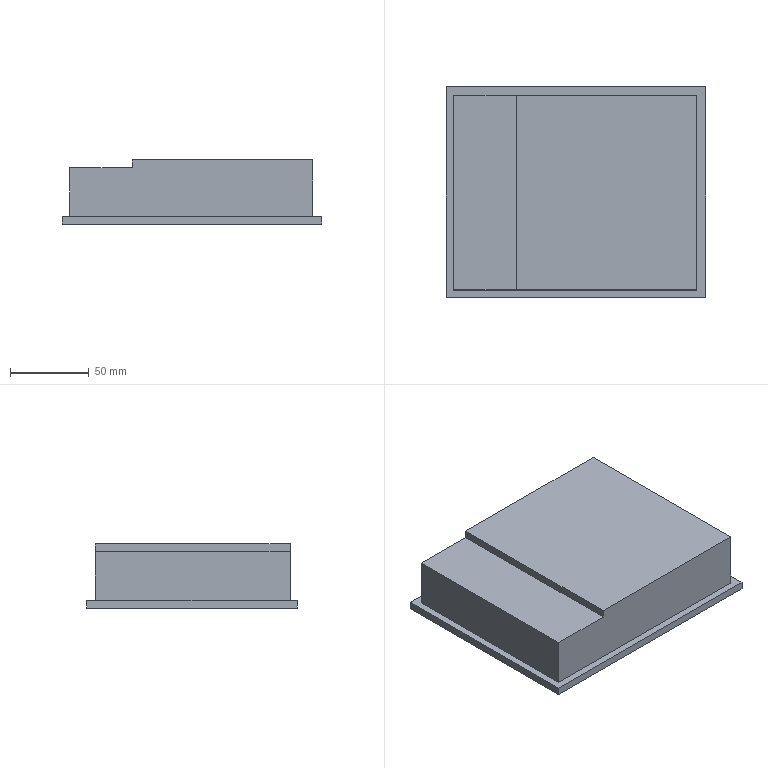Part | STEP file | Display-724_Default | 1 solid | 18 faces | box 165 x 134 x 41 mm | volume 776017 mm3 | plane 18
STEP:
#1=CARTESIAN_POINT('',(0.,0.,0.));
#2=DIRECTION('',(0.,0.,1.));
#3=DIRECTION('',(1.,0.,0.));
#4=AXIS2_PLACEMENT_3D('',#1,#2,#3);
#5=CARTESIAN_POINT('',(-69.492,78.011,5.));
#6=VERTEX_POINT('',#5);
#7=CARTESIAN_POINT('',(-69.492,-55.989,5.));
#8=VERTEX_POINT('',#7);
#9=CARTESIAN_POINT('',(-69.492,78.011,5.));
#10=DIRECTION('',(-0.00000053,-1.,0.));
#11=VECTOR('',#10,1.);
#12=LINE('',#9,#11);
#13=CARTESIAN_POINT('',(-69.492,-55.989,5.));
#14=DIRECTION('',(0.,0.,1.));
#15=DIRECTION('',(1.,0.,0.));
#16=AXIS2_PLACEMENT_3D('',#13,#14,#15);
#17=PLANE('',#16);
#18=CARTESIAN_POINT('',(0.00007096,134.));
#19=DIRECTION('',(-0.00000053,-1.));
#20=VECTOR('',#19,1.);
#21=LINE('',#18,#20);
#22=(GEOMETRIC_REPRESENTATION_CONTEXT(2)PARAMETRIC_REPRESENTATION_CONTEXT()REPRESENTATION_CONTEXT('',''));
#23=DEFINITIONAL_REPRESENTATION('',(#21),#22);
#24=PCURVE('',#17,#23);
#25=CARTESIAN_POINT('',(-69.492,78.011,5.));
#26=DIRECTION('',(1.,-0.00000053,0.));
#27=DIRECTION('',(0.00000053,1.,0.));
#28=AXIS2_PLACEMENT_3D('',#25,#26,#27);
#29=PLANE('',#28);
#30=CARTESIAN_POINT('',(0.,0.));
#31=DIRECTION('',(-1.,0.));
#32=VECTOR('',#31,1.);
#33=LINE('',#30,#32);
#34=(GEOMETRIC_REPRESENTATION_CONTEXT(2)PARAMETRIC_REPRESENTATION_CONTEXT()REPRESENTATION_CONTEXT('',''));
#35=DEFINITIONAL_REPRESENTATION('',(#33),#34);
#36=PCURVE('',#29,#35);
#37=SURFACE_CURVE('',#12,(#24,#36),.PCURVE_S1.);
#38=EDGE_CURVE('',#6,#8,#37,.T.);
#39=ORIENTED_EDGE('',*,*,#38,.T.);
#40=CARTESIAN_POINT('',(95.508,-55.989,5.));
#41=VERTEX_POINT('',#40);
#42=CARTESIAN_POINT('',(-69.492,-55.989,5.));
#43=DIRECTION('',(1.,0.00000006,0.));
#44=VECTOR('',#43,1.);
#45=LINE('',#42,#44);
#46=CARTESIAN_POINT('',(0.,0.));
#47=DIRECTION('',(1.,0.00000006));
#48=VECTOR('',#47,1.);
#49=LINE('',#46,#48);
#50=(GEOMETRIC_REPRESENTATION_CONTEXT(2)PARAMETRIC_REPRESENTATION_CONTEXT()REPRESENTATION_CONTEXT('',''));
#51=DEFINITIONAL_REPRESENTATION('',(#49),#50);
#52=PCURVE('',#17,#51);
#53=CARTESIAN_POINT('',(-69.492,-55.989,5.));
#54=DIRECTION('',(-0.00000006,1.,0.));
#55=DIRECTION('',(-1.,-0.00000006,0.));
#56=AXIS2_PLACEMENT_3D('',#53,#54,#55);
#57=PLANE('',#56);
#58=CARTESIAN_POINT('',(0.,0.));
#59=DIRECTION('',(-1.,0.));
#60=VECTOR('',#59,1.);
#61=LINE('',#58,#60);
#62=(GEOMETRIC_REPRESENTATION_CONTEXT(2)PARAMETRIC_REPRESENTATION_CONTEXT()REPRESENTATION_CONTEXT('',''));
#63=DEFINITIONAL_REPRESENTATION('',(#61),#62);
#64=PCURVE('',#57,#63);
#65=SURFACE_CURVE('',#45,(#52,#64),.PCURVE_S1.);
#66=EDGE_CURVE('',#8,#41,#65,.T.);
#67=ORIENTED_EDGE('',*,*,#66,.T.);
#68=CARTESIAN_POINT('',(95.508,78.011,5.));
#69=VERTEX_POINT('',#68);
#70=CARTESIAN_POINT('',(95.508,78.011,5.));
#71=DIRECTION('',(0.00000053,1.,0.));
#72=VECTOR('',#71,1.);
#73=LINE('',#70,#72);
#74=CARTESIAN_POINT('',(165.,134.));
#75=DIRECTION('',(0.00000053,1.));
#76=VECTOR('',#75,1.);
#77=LINE('',#74,#76);
#78=(GEOMETRIC_REPRESENTATION_CONTEXT(2)PARAMETRIC_REPRESENTATION_CONTEXT()REPRESENTATION_CONTEXT('',''));
#79=DEFINITIONAL_REPRESENTATION('',(#77),#78);
#80=PCURVE('',#17,#79);
#81=CARTESIAN_POINT('',(95.508,78.011,5.));
#82=DIRECTION('',(-1.,0.00000053,0.));
#83=DIRECTION('',(-0.00000053,-1.,0.));
#84=AXIS2_PLACEMENT_3D('',#81,#82,#83);
#85=PLANE('',#84);
#86=CARTESIAN_POINT('',(0.,0.));
#87=DIRECTION('',(-1.,0.));
#88=VECTOR('',#87,1.);
#89=LINE('',#86,#88);
#90=(GEOMETRIC_REPRESENTATION_CONTEXT(2)PARAMETRIC_REPRESENTATION_CONTEXT()REPRESENTATION_CONTEXT('',''));
#91=DEFINITIONAL_REPRESENTATION('',(#89),#90);
#92=PCURVE('',#85,#91);
#93=SURFACE_CURVE('',#73,(#80,#92),.PCURVE_S1.);
#94=EDGE_CURVE('',#41,#69,#93,.T.);
#95=ORIENTED_EDGE('',*,*,#94,.T.);
#96=CARTESIAN_POINT('',(-69.492,78.011,5.));
#97=DIRECTION('',(-1.,-0.00000006,0.));
#98=VECTOR('',#97,1.);
#99=LINE('',#96,#98);
#100=CARTESIAN_POINT('',(0.00007096,134.));
#101=DIRECTION('',(-1.,-0.00000006));
#102=VECTOR('',#101,1.);
#103=LINE('',#100,#102);
#104=(GEOMETRIC_REPRESENTATION_CONTEXT(2)PARAMETRIC_REPRESENTATION_CONTEXT()REPRESENTATION_CONTEXT('',''));
#105=DEFINITIONAL_REPRESENTATION('',(#103),#104);
#106=PCURVE('',#17,#105);
#107=CARTESIAN_POINT('',(-69.492,78.011,5.));
#108=DIRECTION('',(0.00000006,-1.,0.));
#109=DIRECTION('',(1.,0.00000006,0.));
#110=AXIS2_PLACEMENT_3D('',#107,#108,#109);
#111=PLANE('',#110);
#112=CARTESIAN_POINT('',(0.,0.));
#113=DIRECTION('',(-1.,0.));
#114=VECTOR('',#113,1.);
#115=LINE('',#112,#114);
#116=(GEOMETRIC_REPRESENTATION_CONTEXT(2)PARAMETRIC_REPRESENTATION_CONTEXT()REPRESENTATION_CONTEXT('',''));
#117=DEFINITIONAL_REPRESENTATION('',(#115),#116);
#118=PCURVE('',#111,#117);
#119=SURFACE_CURVE('',#99,(#106,#118),.PCURVE_S1.);
#120=EDGE_CURVE('',#69,#6,#119,.T.);
#121=ORIENTED_EDGE('',*,*,#120,.T.);
#122=EDGE_LOOP('',(#39,#67,#95,#121));
#123=FACE_BOUND('',#122,.T.);
#124=CARTESIAN_POINT('',(90.052,72.554,5.));
#125=VERTEX_POINT('',#124);
#126=CARTESIAN_POINT('',(-64.948,72.554,5.));
#127=VERTEX_POINT('',#126);
#128=CARTESIAN_POINT('',(-64.948,72.554,5.));
#129=DIRECTION('',(-1.,0.,0.));
#130=VECTOR('',#129,1.);
#131=LINE('',#128,#130);
#132=CARTESIAN_POINT('',(4.544,128.543));
#133=DIRECTION('',(-1.,0.));
#134=VECTOR('',#133,1.);
#135=LINE('',#132,#134);
#136=(GEOMETRIC_REPRESENTATION_CONTEXT(2)PARAMETRIC_REPRESENTATION_CONTEXT()REPRESENTATION_CONTEXT('',''));
#137=DEFINITIONAL_REPRESENTATION('',(#135),#136);
#138=PCURVE('',#17,#137);
#139=CARTESIAN_POINT('',(-64.948,72.554,41.));
#140=DIRECTION('',(0.,-1.,0.));
#141=DIRECTION('',(0.,0.,-1.));
#142=AXIS2_PLACEMENT_3D('',#139,#140,#141);
#143=PLANE('',#142);
#144=CARTESIAN_POINT('',(36.,0.));
#145=DIRECTION('',(0.,-1.));
#146=VECTOR('',#145,1.);
#147=LINE('',#144,#146);
#148=(GEOMETRIC_REPRESENTATION_CONTEXT(2)PARAMETRIC_REPRESENTATION_CONTEXT()REPRESENTATION_CONTEXT('',''));
#149=DEFINITIONAL_REPRESENTATION('',(#147),#148);
#150=PCURVE('',#143,#149);
#151=SURFACE_CURVE('',#131,(#138,#150),.PCURVE_S1.);
#152=EDGE_CURVE('',#125,#127,#151,.T.);
#153=ORIENTED_EDGE('',*,*,#152,.F.);
#154=CARTESIAN_POINT('',(90.052,-51.446,5.));
#155=VERTEX_POINT('',#154);
#156=CARTESIAN_POINT('',(90.052,72.554,5.));
#157=DIRECTION('',(0.,1.,0.));
#158=VECTOR('',#157,1.);
#159=LINE('',#156,#158);
#160=CARTESIAN_POINT('',(159.544,128.543));
#161=DIRECTION('',(0.,1.));
#162=VECTOR('',#161,1.);
#163=LINE('',#160,#162);
#164=(GEOMETRIC_REPRESENTATION_CONTEXT(2)PARAMETRIC_REPRESENTATION_CONTEXT()REPRESENTATION_CONTEXT('',''));
#165=DEFINITIONAL_REPRESENTATION('',(#163),#164);
#166=PCURVE('',#17,#165);
#167=CARTESIAN_POINT('',(90.052,72.554,41.));
#168=DIRECTION('',(-1.,0.,0.));
#169=DIRECTION('',(0.,-1.,0.));
#170=AXIS2_PLACEMENT_3D('',#167,#168,#169);
#171=PLANE('',#170);
#172=CARTESIAN_POINT('',(0.,-36.));
#173=DIRECTION('',(-1.,0.));
#174=VECTOR('',#173,1.);
#175=LINE('',#172,#174);
#176=(GEOMETRIC_REPRESENTATION_CONTEXT(2)PARAMETRIC_REPRESENTATION_CONTEXT()REPRESENTATION_CONTEXT('',''));
#177=DEFINITIONAL_REPRESENTATION('',(#175),#176);
#178=PCURVE('',#171,#177);
#179=SURFACE_CURVE('',#159,(#166,#178),.PCURVE_S1.);
#180=EDGE_CURVE('',#155,#125,#179,.T.);
#181=ORIENTED_EDGE('',*,*,#180,.F.);
#182=CARTESIAN_POINT('',(-64.948,-51.446,5.));
#183=VERTEX_POINT('',#182);
#184=CARTESIAN_POINT('',(-64.948,-51.446,5.));
#185=DIRECTION('',(1.,0.,0.));
#186=VECTOR('',#185,1.);
#187=LINE('',#184,#186);
#188=CARTESIAN_POINT('',(4.544,4.543));
#189=DIRECTION('',(1.,0.));
#190=VECTOR('',#189,1.);
#191=LINE('',#188,#190);
#192=(GEOMETRIC_REPRESENTATION_CONTEXT(2)PARAMETRIC_REPRESENTATION_CONTEXT()REPRESENTATION_CONTEXT('',''));
#193=DEFINITIONAL_REPRESENTATION('',(#191),#192);
#194=PCURVE('',#17,#193);
#195=CARTESIAN_POINT('',(-64.948,-51.446,41.));
#196=DIRECTION('',(0.,1.,0.));
#197=DIRECTION('',(0.,0.,1.));
#198=AXIS2_PLACEMENT_3D('',#195,#196,#197);
#199=PLANE('',#198);
#200=CARTESIAN_POINT('',(-36.,0.));
#201=DIRECTION('',(0.,1.));
#202=VECTOR('',#201,1.);
#203=LINE('',#200,#202);
#204=(GEOMETRIC_REPRESENTATION_CONTEXT(2)PARAMETRIC_REPRESENTATION_CONTEXT()REPRESENTATION_CONTEXT('',''));
#205=DEFINITIONAL_REPRESENTATION('',(#203),#204);
#206=PCURVE('',#199,#205);
#207=SURFACE_CURVE('',#187,(#194,#206),.PCURVE_S1.);
#208=EDGE_CURVE('',#183,#155,#207,.T.);
#209=ORIENTED_EDGE('',*,*,#208,.F.);
#210=CARTESIAN_POINT('',(-64.948,72.554,5.));
#211=DIRECTION('',(0.,-1.,0.));
#212=VECTOR('',#211,1.);
#213=LINE('',#210,#212);
#214=CARTESIAN_POINT('',(4.544,128.543));
#215=DIRECTION('',(0.,-1.));
#216=VECTOR('',#215,1.);
#217=LINE('',#214,#216);
#218=(GEOMETRIC_REPRESENTATION_CONTEXT(2)PARAMETRIC_REPRESENTATION_CONTEXT()REPRESENTATION_CONTEXT('',''));
#219=DEFINITIONAL_REPRESENTATION('',(#217),#218);
#220=PCURVE('',#17,#219);
#221=CARTESIAN_POINT('',(-64.948,72.554,41.));
#222=DIRECTION('',(1.,0.,0.));
#223=DIRECTION('',(0.,1.,0.));
#224=AXIS2_PLACEMENT_3D('',#221,#222,#223);
#225=PLANE('',#224);
#226=CARTESIAN_POINT('',(0.,-36.));
#227=DIRECTION('',(-1.,0.));
#228=VECTOR('',#227,1.);
#229=LINE('',#226,#228);
#230=(GEOMETRIC_REPRESENTATION_CONTEXT(2)PARAMETRIC_REPRESENTATION_CONTEXT()REPRESENTATION_CONTEXT('',''));
#231=DEFINITIONAL_REPRESENTATION('',(#229),#230);
#232=PCURVE('',#225,#231);
#233=SURFACE_CURVE('',#213,(#220,#232),.PCURVE_S1.);
#234=EDGE_CURVE('',#127,#183,#233,.T.);
#235=ORIENTED_EDGE('',*,*,#234,.F.);
#236=EDGE_LOOP('',(#153,#181,#209,#235));
#237=FACE_BOUND('',#236,.T.);
#238=ADVANCED_FACE('',(#123,#237),#17,.T.);
#239=CARTESIAN_POINT('',(-69.492,78.011,0.));
#240=VERTEX_POINT('',#239);
#241=CARTESIAN_POINT('',(-69.492,-55.989,0.));
#242=VERTEX_POINT('',#241);
#243=CARTESIAN_POINT('',(-69.492,78.011,0.));
#244=DIRECTION('',(-0.00000053,-1.,0.));
#245=VECTOR('',#244,1.);
#246=LINE('',#243,#245);
#247=CARTESIAN_POINT('',(0.,-5.));
#248=DIRECTION('',(-1.,0.));
#249=VECTOR('',#248,1.);
#250=LINE('',#247,#249);
#251=(GEOMETRIC_REPRESENTATION_CONTEXT(2)PARAMETRIC_REPRESENTATION_CONTEXT()REPRESENTATION_CONTEXT('',''));
#252=DEFINITIONAL_REPRESENTATION('',(#250),#251);
#253=PCURVE('',#29,#252);
#254=CARTESIAN_POINT('',(-69.492,-55.989,0.));
#255=DIRECTION('',(0.,0.,1.));
#256=DIRECTION('',(1.,0.,0.));
#257=AXIS2_PLACEMENT_3D('',#254,#255,#256);
#258=PLANE('',#257);
#259=CARTESIAN_POINT('',(0.00007096,134.));
#260=DIRECTION('',(-0.00000053,-1.));
#261=VECTOR('',#260,1.);
#262=LINE('',#259,#261);
#263=(GEOMETRIC_REPRESENTATION_CONTEXT(2)PARAMETRIC_REPRESENTATION_CONTEXT()REPRESENTATION_CONTEXT('',''));
#264=DEFINITIONAL_REPRESENTATION('',(#262),#263);
#265=PCURVE('',#258,#264);
#266=SURFACE_CURVE('',#246,(#253,#265),.PCURVE_S1.);
#267=EDGE_CURVE('',#240,#242,#266,.T.);
#268=ORIENTED_EDGE('',*,*,#267,.T.);
#269=CARTESIAN_POINT('',(-69.492,-55.989,5.));
#270=DIRECTION('',(0.,0.,-1.));
#271=VECTOR('',#270,1.);
#272=LINE('',#269,#271);
#273=CARTESIAN_POINT('',(-134.,0.));
#274=DIRECTION('',(0.,-1.));
#275=VECTOR('',#274,1.);
#276=LINE('',#273,#275);
#277=(GEOMETRIC_REPRESENTATION_CONTEXT(2)PARAMETRIC_REPRESENTATION_CONTEXT()REPRESENTATION_CONTEXT('',''));
#278=DEFINITIONAL_REPRESENTATION('',(#276),#277);
#279=PCURVE('',#29,#278);
#280=CARTESIAN_POINT('',(0.,0.));
#281=DIRECTION('',(0.,-1.));
#282=VECTOR('',#281,1.);
#283=LINE('',#280,#282);
#284=(GEOMETRIC_REPRESENTATION_CONTEXT(2)PARAMETRIC_REPRESENTATION_CONTEXT()REPRESENTATION_CONTEXT('',''));
#285=DEFINITIONAL_REPRESENTATION('',(#283),#284);
#286=PCURVE('',#57,#285);
#287=SURFACE_CURVE('',#272,(#279,#286),.PCURVE_S1.);
#288=EDGE_CURVE('',#8,#242,#287,.T.);
#289=ORIENTED_EDGE('',*,*,#288,.F.);
#290=ORIENTED_EDGE('',*,*,#38,.F.);
#291=CARTESIAN_POINT('',(-69.492,78.011,5.));
#292=DIRECTION('',(0.,0.,-1.));
#293=VECTOR('',#292,1.);
#294=LINE('',#291,#293);
#295=CARTESIAN_POINT('',(0.,0.));
#296=DIRECTION('',(0.,-1.));
#297=VECTOR('',#296,1.);
#298=LINE('',#295,#297);
#299=(GEOMETRIC_REPRESENTATION_CONTEXT(2)PARAMETRIC_REPRESENTATION_CONTEXT()REPRESENTATION_CONTEXT('',''));
#300=DEFINITIONAL_REPRESENTATION('',(#298),#299);
#301=PCURVE('',#29,#300);
#302=CARTESIAN_POINT('',(0.,0.));
#303=DIRECTION('',(0.,-1.));
#304=VECTOR('',#303,1.);
#305=LINE('',#302,#304);
#306=(GEOMETRIC_REPRESENTATION_CONTEXT(2)PARAMETRIC_REPRESENTATION_CONTEXT()REPRESENTATION_CONTEXT('',''));
#307=DEFINITIONAL_REPRESENTATION('',(#305),#306);
#308=PCURVE('',#111,#307);
#309=SURFACE_CURVE('',#294,(#301,#308),.PCURVE_S1.);
#310=EDGE_CURVE('',#6,#240,#309,.T.);
#311=ORIENTED_EDGE('',*,*,#310,.T.);
#312=EDGE_LOOP('',(#268,#289,#290,#311));
#313=FACE_BOUND('',#312,.T.);
#314=ADVANCED_FACE('',(#313),#29,.F.);
#315=CARTESIAN_POINT('',(95.508,-55.989,0.));
#316=VERTEX_POINT('',#315);
#317=CARTESIAN_POINT('',(-69.492,-55.989,0.));
#318=DIRECTION('',(1.,0.00000006,0.));
#319=VECTOR('',#318,1.);
#320=LINE('',#317,#319);
#321=CARTESIAN_POINT('',(0.,-5.));
#322=DIRECTION('',(-1.,0.));
#323=VECTOR('',#322,1.);
#324=LINE('',#321,#323);
#325=(GEOMETRIC_REPRESENTATION_CONTEXT(2)PARAMETRIC_REPRESENTATION_CONTEXT()REPRESENTATION_CONTEXT('',''));
#326=DEFINITIONAL_REPRESENTATION('',(#324),#325);
#327=PCURVE('',#57,#326);
#328=CARTESIAN_POINT('',(0.,0.));
#329=DIRECTION('',(1.,0.00000006));
#330=VECTOR('',#329,1.);
#331=LINE('',#328,#330);
#332=(GEOMETRIC_REPRESENTATION_CONTEXT(2)PARAMETRIC_REPRESENTATION_CONTEXT()REPRESENTATION_CONTEXT('',''));
#333=DEFINITIONAL_REPRESENTATION('',(#331),#332);
#334=PCURVE('',#258,#333);
#335=SURFACE_CURVE('',#320,(#327,#334),.PCURVE_S1.);
#336=EDGE_CURVE('',#242,#316,#335,.T.);
#337=ORIENTED_EDGE('',*,*,#336,.T.);
#338=CARTESIAN_POINT('',(95.508,-55.989,5.));
#339=DIRECTION('',(0.,0.,-1.));
#340=VECTOR('',#339,1.);
#341=LINE('',#338,#340);
#342=CARTESIAN_POINT('',(-165.,0.));
#343=DIRECTION('',(0.,-1.));
#344=VECTOR('',#343,1.);
#345=LINE('',#342,#344);
#346=(GEOMETRIC_REPRESENTATION_CONTEXT(2)PARAMETRIC_REPRESENTATION_CONTEXT()REPRESENTATION_CONTEXT('',''));
#347=DEFINITIONAL_REPRESENTATION('',(#345),#346);
#348=PCURVE('',#57,#347);
#349=CARTESIAN_POINT('',(134.,0.));
#350=DIRECTION('',(0.,-1.));
#351=VECTOR('',#350,1.);
#352=LINE('',#349,#351);
#353=(GEOMETRIC_REPRESENTATION_CONTEXT(2)PARAMETRIC_REPRESENTATION_CONTEXT()REPRESENTATION_CONTEXT('',''));
#354=DEFINITIONAL_REPRESENTATION('',(#352),#353);
#355=PCURVE('',#85,#354);
#356=SURFACE_CURVE('',#341,(#348,#355),.PCURVE_S1.);
#357=EDGE_CURVE('',#41,#316,#356,.T.);
#358=ORIENTED_EDGE('',*,*,#357,.F.);
#359=ORIENTED_EDGE('',*,*,#66,.F.);
#360=ORIENTED_EDGE('',*,*,#288,.T.);
#361=EDGE_LOOP('',(#337,#358,#359,#360));
#362=FACE_BOUND('',#361,.T.);
#363=ADVANCED_FACE('',(#362),#57,.F.);
#364=CARTESIAN_POINT('',(95.508,78.011,0.));
#365=VERTEX_POINT('',#364);
#366=CARTESIAN_POINT('',(95.508,78.011,0.));
#367=DIRECTION('',(0.00000053,1.,0.));
#368=VECTOR('',#367,1.);
#369=LINE('',#366,#368);
#370=CARTESIAN_POINT('',(0.,-5.));
#371=DIRECTION('',(-1.,0.));
#372=VECTOR('',#371,1.);
#373=LINE('',#370,#372);
#374=(GEOMETRIC_REPRESENTATION_CONTEXT(2)PARAMETRIC_REPRESENTATION_CONTEXT()REPRESENTATION_CONTEXT('',''));
#375=DEFINITIONAL_REPRESENTATION('',(#373),#374);
#376=PCURVE('',#85,#375);
#377=CARTESIAN_POINT('',(165.,134.));
#378=DIRECTION('',(0.00000053,1.));
#379=VECTOR('',#378,1.);
#380=LINE('',#377,#379);
#381=(GEOMETRIC_REPRESENTATION_CONTEXT(2)PARAMETRIC_REPRESENTATION_CONTEXT()REPRESENTATION_CONTEXT('',''));
#382=DEFINITIONAL_REPRESENTATION('',(#380),#381);
#383=PCURVE('',#258,#382);
#384=SURFACE_CURVE('',#369,(#376,#383),.PCURVE_S1.);
#385=EDGE_CURVE('',#316,#365,#384,.T.);
#386=ORIENTED_EDGE('',*,*,#385,.T.);
#387=CARTESIAN_POINT('',(95.508,78.011,5.));
#388=DIRECTION('',(0.,0.,-1.));
#389=VECTOR('',#388,1.);
#390=LINE('',#387,#389);
#391=CARTESIAN_POINT('',(0.,0.));
#392=DIRECTION('',(0.,-1.));
#393=VECTOR('',#392,1.);
#394=LINE('',#391,#393);
#395=(GEOMETRIC_REPRESENTATION_CONTEXT(2)PARAMETRIC_REPRESENTATION_CONTEXT()REPRESENTATION_CONTEXT('',''));
#396=DEFINITIONAL_REPRESENTATION('',(#394),#395);
#397=PCURVE('',#85,#396);
#398=CARTESIAN_POINT('',(165.,0.));
#399=DIRECTION('',(0.,-1.));
#400=VECTOR('',#399,1.);
#401=LINE('',#398,#400);
#402=(GEOMETRIC_REPRESENTATION_CONTEXT(2)PARAMETRIC_REPRESENTATION_CONTEXT()REPRESENTATION_CONTEXT('',''));
#403=DEFINITIONAL_REPRESENTATION('',(#401),#402);
#404=PCURVE('',#111,#403);
#405=SURFACE_CURVE('',#390,(#397,#404),.PCURVE_S1.);
#406=EDGE_CURVE('',#69,#365,#405,.T.);
#407=ORIENTED_EDGE('',*,*,#406,.F.);
#408=ORIENTED_EDGE('',*,*,#94,.F.);
#409=ORIENTED_EDGE('',*,*,#357,.T.);
#410=EDGE_LOOP('',(#386,#407,#408,#409));
#411=FACE_BOUND('',#410,.T.);
#412=ADVANCED_FACE('',(#411),#85,.F.);
#413=CARTESIAN_POINT('',(-69.492,78.011,0.));
#414=DIRECTION('',(-1.,-0.00000006,0.));
#415=VECTOR('',#414,1.);
#416=LINE('',#413,#415);
#417=CARTESIAN_POINT('',(0.,-5.));
#418=DIRECTION('',(-1.,0.));
#419=VECTOR('',#418,1.);
#420=LINE('',#417,#419);
#421=(GEOMETRIC_REPRESENTATION_CONTEXT(2)PARAMETRIC_REPRESENTATION_CONTEXT()REPRESENTATION_CONTEXT('',''));
#422=DEFINITIONAL_REPRESENTATION('',(#420),#421);
#423=PCURVE('',#111,#422);
#424=CARTESIAN_POINT('',(0.00007096,134.));
#425=DIRECTION('',(-1.,-0.00000006));
#426=VECTOR('',#425,1.);
#427=LINE('',#424,#426);
#428=(GEOMETRIC_REPRESENTATION_CONTEXT(2)PARAMETRIC_REPRESENTATION_CONTEXT()REPRESENTATION_CONTEXT('',''));
#429=DEFINITIONAL_REPRESENTATION('',(#427),#428);
#430=PCURVE('',#258,#429);
#431=SURFACE_CURVE('',#416,(#423,#430),.PCURVE_S1.);
#432=EDGE_CURVE('',#365,#240,#431,.T.);
#433=ORIENTED_EDGE('',*,*,#432,.T.);
#434=ORIENTED_EDGE('',*,*,#310,.F.);
#435=ORIENTED_EDGE('',*,*,#120,.F.);
#436=ORIENTED_EDGE('',*,*,#406,.T.);
#437=EDGE_LOOP('',(#433,#434,#435,#436));
#438=FACE_BOUND('',#437,.T.);
#439=ADVANCED_FACE('',(#438),#111,.F.);
#440=CARTESIAN_POINT('',(85.508,-45.989,0.));
#441=VERTEX_POINT('',#440);
#442=CARTESIAN_POINT('',(-59.492,-45.989,0.));
#443=VERTEX_POINT('',#442);
#444=CARTESIAN_POINT('',(85.508,-45.989,0.));
#445=DIRECTION('',(-1.,-0.00000006,0.));
#446=VECTOR('',#445,1.);
#447=LINE('',#444,#446);
#448=CARTESIAN_POINT('',(155.,10.));
#449=DIRECTION('',(-1.,-0.00000006));
#450=VECTOR('',#449,1.);
#451=LINE('',#448,#450);
#452=(GEOMETRIC_REPRESENTATION_CONTEXT(2)PARAMETRIC_REPRESENTATION_CONTEXT()REPRESENTATION_CONTEXT('',''));
#453=DEFINITIONAL_REPRESENTATION('',(#451),#452);
#454=PCURVE('',#258,#453);
#455=CARTESIAN_POINT('',(85.508,-45.989,0.1));
#456=DIRECTION('',(0.00000006,-1.,0.));
#457=DIRECTION('',(1.,0.00000006,0.));
#458=AXIS2_PLACEMENT_3D('',#455,#456,#457);
#459=PLANE('',#458);
#460=CARTESIAN_POINT('',(0.,-0.1));
#461=DIRECTION('',(-1.,0.));
#462=VECTOR('',#461,1.);
#463=LINE('',#460,#462);
#464=(GEOMETRIC_REPRESENTATION_CONTEXT(2)PARAMETRIC_REPRESENTATION_CONTEXT()REPRESENTATION_CONTEXT('',''));
#465=DEFINITIONAL_REPRESENTATION('',(#463),#464);
#466=PCURVE('',#459,#465);
#467=SURFACE_CURVE('',#447,(#454,#466),.PCURVE_S1.);
#468=EDGE_CURVE('',#441,#443,#467,.T.);
#469=ORIENTED_EDGE('',*,*,#468,.F.);
#470=CARTESIAN_POINT('',(85.508,68.011,0.));
#471=VERTEX_POINT('',#470);
#472=CARTESIAN_POINT('',(85.508,68.011,0.));
#473=DIRECTION('',(-0.00000053,-1.,0.));
#474=VECTOR('',#473,1.);
#475=LINE('',#472,#474);
#476=CARTESIAN_POINT('',(155.,124.));
#477=DIRECTION('',(-0.00000053,-1.));
#478=VECTOR('',#477,1.);
#479=LINE('',#476,#478);
#480=(GEOMETRIC_REPRESENTATION_CONTEXT(2)PARAMETRIC_REPRESENTATION_CONTEXT()REPRESENTATION_CONTEXT('',''));
#481=DEFINITIONAL_REPRESENTATION('',(#479),#480);
#482=PCURVE('',#258,#481);
#483=CARTESIAN_POINT('',(85.508,68.011,0.1));
#484=DIRECTION('',(1.,-0.00000053,0.));
#485=DIRECTION('',(0.00000053,1.,0.));
#486=AXIS2_PLACEMENT_3D('',#483,#484,#485);
#487=PLANE('',#486);
#488=CARTESIAN_POINT('',(0.,-0.1));
#489=DIRECTION('',(-1.,0.));
#490=VECTOR('',#489,1.);
#491=LINE('',#488,#490);
#492=(GEOMETRIC_REPRESENTATION_CONTEXT(2)PARAMETRIC_REPRESENTATION_CONTEXT()REPRESENTATION_CONTEXT('',''));
#493=DEFINITIONAL_REPRESENTATION('',(#491),#492);
#494=PCURVE('',#487,#493);
#495=SURFACE_CURVE('',#475,(#482,#494),.PCURVE_S1.);
#496=EDGE_CURVE('',#471,#441,#495,.T.);
#497=ORIENTED_EDGE('',*,*,#496,.F.);
#498=CARTESIAN_POINT('',(-59.492,68.011,0.));
#499=VERTEX_POINT('',#498);
#500=CARTESIAN_POINT('',(85.508,68.011,0.));
#501=DIRECTION('',(1.,0.00000006,0.));
#502=VECTOR('',#501,1.);
#503=LINE('',#500,#502);
#504=CARTESIAN_POINT('',(155.,124.));
#505=DIRECTION('',(1.,0.00000006));
#506=VECTOR('',#505,1.);
#507=LINE('',#504,#506);
#508=(GEOMETRIC_REPRESENTATION_CONTEXT(2)PARAMETRIC_REPRESENTATION_CONTEXT()REPRESENTATION_CONTEXT('',''));
#509=DEFINITIONAL_REPRESENTATION('',(#507),#508);
#510=PCURVE('',#258,#509);
#511=CARTESIAN_POINT('',(85.508,68.011,0.1));
#512=DIRECTION('',(-0.00000006,1.,0.));
#513=DIRECTION('',(-1.,-0.00000006,0.));
#514=AXIS2_PLACEMENT_3D('',#511,#512,#513);
#515=PLANE('',#514);
#516=CARTESIAN_POINT('',(0.,-0.1));
#517=DIRECTION('',(-1.,0.));
#518=VECTOR('',#517,1.);
#519=LINE('',#516,#518);
#520=(GEOMETRIC_REPRESENTATION_CONTEXT(2)PARAMETRIC_REPRESENTATION_CONTEXT()REPRESENTATION_CONTEXT('',''));
#521=DEFINITIONAL_REPRESENTATION('',(#519),#520);
#522=PCURVE('',#515,#521);
#523=SURFACE_CURVE('',#503,(#510,#522),.PCURVE_S1.);
#524=EDGE_CURVE('',#499,#471,#523,.T.);
#525=ORIENTED_EDGE('',*,*,#524,.F.);
#526=CARTESIAN_POINT('',(-59.492,68.011,0.));
#527=DIRECTION('',(0.00000053,1.,0.));
#528=VECTOR('',#527,1.);
#529=LINE('',#526,#528);
#530=CARTESIAN_POINT('',(10.,124.));
#531=DIRECTION('',(0.00000053,1.));
#532=VECTOR('',#531,1.);
#533=LINE('',#530,#532);
#534=(GEOMETRIC_REPRESENTATION_CONTEXT(2)PARAMETRIC_REPRESENTATION_CONTEXT()REPRESENTATION_CONTEXT('',''));
#535=DEFINITIONAL_REPRESENTATION('',(#533),#534);
#536=PCURVE('',#258,#535);
#537=CARTESIAN_POINT('',(-59.492,68.011,0.1));
#538=DIRECTION('',(-1.,0.00000053,0.));
#539=DIRECTION('',(-0.00000053,-1.,0.));
#540=AXIS2_PLACEMENT_3D('',#537,#538,#539);
#541=PLANE('',#540);
#542=CARTESIAN_POINT('',(0.,-0.1));
#543=DIRECTION('',(-1.,0.));
#544=VECTOR('',#543,1.);
#545=LINE('',#542,#544);
#546=(GEOMETRIC_REPRESENTATION_CONTEXT(2)PARAMETRIC_REPRESENTATION_CONTEXT()REPRESENTATION_CONTEXT('',''));
#547=DEFINITIONAL_REPRESENTATION('',(#545),#546);
#548=PCURVE('',#541,#547);
#549=SURFACE_CURVE('',#529,(#536,#548),.PCURVE_S1.);
#550=EDGE_CURVE('',#443,#499,#549,.T.);
#551=ORIENTED_EDGE('',*,*,#550,.F.);
#552=EDGE_LOOP('',(#469,#497,#525,#551));
#553=FACE_BOUND('',#552,.T.);
#554=ORIENTED_EDGE('',*,*,#267,.F.);
#555=ORIENTED_EDGE('',*,*,#432,.F.);
#556=ORIENTED_EDGE('',*,*,#385,.F.);
#557=ORIENTED_EDGE('',*,*,#336,.F.);
#558=EDGE_LOOP('',(#554,#555,#556,#557));
#559=FACE_BOUND('',#558,.T.);
#560=ADVANCED_FACE('',(#553,#559),#258,.F.);
#561=ORIENTED_EDGE('',*,*,#180,.T.);
#562=CARTESIAN_POINT('',(90.052,72.554,41.));
#563=VERTEX_POINT('',#562);
#564=CARTESIAN_POINT('',(90.052,72.554,41.));
#565=DIRECTION('',(0.,0.,-1.));
#566=VECTOR('',#565,1.);
#567=LINE('',#564,#566);
#568=CARTESIAN_POINT('',(0.,0.));
#569=DIRECTION('',(0.,-1.));
#570=VECTOR('',#569,1.);
#571=LINE('',#568,#570);
#572=(GEOMETRIC_REPRESENTATION_CONTEXT(2)PARAMETRIC_REPRESENTATION_CONTEXT()REPRESENTATION_CONTEXT('',''));
#573=DEFINITIONAL_REPRESENTATION('',(#571),#572);
#574=PCURVE('',#171,#573);
#575=CARTESIAN_POINT('',(0.,155.));
#576=DIRECTION('',(1.,0.));
#577=VECTOR('',#576,1.);
#578=LINE('',#575,#577);
#579=(GEOMETRIC_REPRESENTATION_CONTEXT(2)PARAMETRIC_REPRESENTATION_CONTEXT()REPRESENTATION_CONTEXT('',''));
#580=DEFINITIONAL_REPRESENTATION('',(#578),#579);
#581=PCURVE('',#143,#580);
#582=SURFACE_CURVE('',#567,(#574,#581),.PCURVE_S1.);
#583=EDGE_CURVE('',#563,#125,#582,.T.);
#584=ORIENTED_EDGE('',*,*,#583,.F.);
#585=CARTESIAN_POINT('',(90.052,-51.446,41.));
#586=VERTEX_POINT('',#585);
#587=CARTESIAN_POINT('',(90.052,72.554,41.));
#588=DIRECTION('',(0.,1.,0.));
#589=VECTOR('',#588,1.);
#590=LINE('',#587,#589);
#591=CARTESIAN_POINT('',(0.,0.));
#592=DIRECTION('',(-1.,0.));
#593=VECTOR('',#592,1.);
#594=LINE('',#591,#593);
#595=(GEOMETRIC_REPRESENTATION_CONTEXT(2)PARAMETRIC_REPRESENTATION_CONTEXT()REPRESENTATION_CONTEXT('',''));
#596=DEFINITIONAL_REPRESENTATION('',(#594),#595);
#597=PCURVE('',#171,#596);
#598=CARTESIAN_POINT('',(90.052,-51.446,41.));
#599=DIRECTION('',(0.,0.,1.));
#600=DIRECTION('',(1.,0.,0.));
#601=AXIS2_PLACEMENT_3D('',#598,#599,#600);
#602=PLANE('',#601);
#603=CARTESIAN_POINT('',(0.,124.));
#604=DIRECTION('',(0.,1.));
#605=VECTOR('',#604,1.);
#606=LINE('',#603,#605);
#607=(GEOMETRIC_REPRESENTATION_CONTEXT(2)PARAMETRIC_REPRESENTATION_CONTEXT()REPRESENTATION_CONTEXT('',''));
#608=DEFINITIONAL_REPRESENTATION('',(#606),#607);
#609=PCURVE('',#602,#608);
#610=SURFACE_CURVE('',#590,(#597,#609),.PCURVE_S1.);
#611=EDGE_CURVE('',#586,#563,#610,.T.);
#612=ORIENTED_EDGE('',*,*,#611,.F.);
#613=CARTESIAN_POINT('',(90.052,-51.446,41.));
#614=DIRECTION('',(0.,0.,-1.));
#615=VECTOR('',#614,1.);
#616=LINE('',#613,#615);
#617=CARTESIAN_POINT('',(124.,0.));
#618=DIRECTION('',(0.,-1.));
#619=VECTOR('',#618,1.);
#620=LINE('',#617,#619);
#621=(GEOMETRIC_REPRESENTATION_CONTEXT(2)PARAMETRIC_REPRESENTATION_CONTEXT()REPRESENTATION_CONTEXT('',''));
#622=DEFINITIONAL_REPRESENTATION('',(#620),#621);
#623=PCURVE('',#171,#622);
#624=CARTESIAN_POINT('',(0.,155.));
#625=DIRECTION('',(-1.,0.));
#626=VECTOR('',#625,1.);
#627=LINE('',#624,#626);
#628=(GEOMETRIC_REPRESENTATION_CONTEXT(2)PARAMETRIC_REPRESENTATION_CONTEXT()REPRESENTATION_CONTEXT('',''));
#629=DEFINITIONAL_REPRESENTATION('',(#627),#628);
#630=PCURVE('',#199,#629);
#631=SURFACE_CURVE('',#616,(#623,#630),.PCURVE_S1.);
#632=EDGE_CURVE('',#586,#155,#631,.T.);
#633=ORIENTED_EDGE('',*,*,#632,.T.);
#634=EDGE_LOOP('',(#561,#584,#612,#633));
#635=FACE_BOUND('',#634,.T.);
#636=ADVANCED_FACE('',(#635),#171,.F.);
#637=CARTESIAN_POINT('',(-24.948,72.554,36.));
#638=VERTEX_POINT('',#637);
#639=CARTESIAN_POINT('',(-64.948,72.554,36.));
#640=VERTEX_POINT('',#639);
#641=CARTESIAN_POINT('',(-91.166,72.554,36.));
#642=DIRECTION('',(-1.,0.,0.));
#643=VECTOR('',#642,1.);
#644=LINE('',#641,#643);
#645=CARTESIAN_POINT('',(5.,-26.217));
#646=DIRECTION('',(0.,-1.));
#647=VECTOR('',#646,1.);
#648=LINE('',#645,#647);
#649=(GEOMETRIC_REPRESENTATION_CONTEXT(2)PARAMETRIC_REPRESENTATION_CONTEXT()REPRESENTATION_CONTEXT('',''));
#650=DEFINITIONAL_REPRESENTATION('',(#648),#649);
#651=PCURVE('',#143,#650);
#652=CARTESIAN_POINT('',(-91.166,-56.446,36.));
#653=DIRECTION('',(0.,0.,-1.));
#654=DIRECTION('',(-1.,0.,0.));
#655=AXIS2_PLACEMENT_3D('',#652,#653,#654);
#656=PLANE('',#655);
#657=CARTESIAN_POINT('',(0.,129.));
#658=DIRECTION('',(1.,0.));
#659=VECTOR('',#658,1.);
#660=LINE('',#657,#659);
#661=(GEOMETRIC_REPRESENTATION_CONTEXT(2)PARAMETRIC_REPRESENTATION_CONTEXT()REPRESENTATION_CONTEXT('',''));
#662=DEFINITIONAL_REPRESENTATION('',(#660),#661);
#663=PCURVE('',#656,#662);
#664=SURFACE_CURVE('',#644,(#651,#663),.PCURVE_S1.);
#665=EDGE_CURVE('',#638,#640,#664,.T.);
#666=ORIENTED_EDGE('',*,*,#665,.F.);
#667=CARTESIAN_POINT('',(-24.948,72.554,41.));
#668=VERTEX_POINT('',#667);
#669=CARTESIAN_POINT('',(-24.948,72.554,36.));
#670=DIRECTION('',(0.,0.,-1.));
#671=VECTOR('',#670,1.);
#672=LINE('',#669,#671);
#673=CARTESIAN_POINT('',(5.,40.));
#674=DIRECTION('',(1.,0.));
#675=VECTOR('',#674,1.);
#676=LINE('',#673,#675);
#677=(GEOMETRIC_REPRESENTATION_CONTEXT(2)PARAMETRIC_REPRESENTATION_CONTEXT()REPRESENTATION_CONTEXT('',''));
#678=DEFINITIONAL_REPRESENTATION('',(#676),#677);
#679=PCURVE('',#143,#678);
#680=CARTESIAN_POINT('',(-24.948,-56.446,36.));
#681=DIRECTION('',(1.,0.,0.));
#682=DIRECTION('',(0.,0.,-1.));
#683=AXIS2_PLACEMENT_3D('',#680,#681,#682);
#684=PLANE('',#683);
#685=CARTESIAN_POINT('',(0.,129.));
#686=DIRECTION('',(1.,0.));
#687=VECTOR('',#686,1.);
#688=LINE('',#685,#687);
#689=(GEOMETRIC_REPRESENTATION_CONTEXT(2)PARAMETRIC_REPRESENTATION_CONTEXT()REPRESENTATION_CONTEXT('',''));
#690=DEFINITIONAL_REPRESENTATION('',(#688),#689);
#691=PCURVE('',#684,#690);
#692=SURFACE_CURVE('',#672,(#679,#691),.PCURVE_S1.);
#693=EDGE_CURVE('',#668,#638,#692,.T.);
#694=ORIENTED_EDGE('',*,*,#693,.F.);
#695=CARTESIAN_POINT('',(-64.948,72.554,41.));
#696=DIRECTION('',(-1.,0.,0.));
#697=VECTOR('',#696,1.);
#698=LINE('',#695,#697);
#699=CARTESIAN_POINT('',(0.,0.));
#700=DIRECTION('',(0.,-1.));
#701=VECTOR('',#700,1.);
#702=LINE('',#699,#701);
#703=(GEOMETRIC_REPRESENTATION_CONTEXT(2)PARAMETRIC_REPRESENTATION_CONTEXT()REPRESENTATION_CONTEXT('',''));
#704=DEFINITIONAL_REPRESENTATION('',(#702),#703);
#705=PCURVE('',#143,#704);
#706=CARTESIAN_POINT('',(-155.,124.));
#707=DIRECTION('',(-1.,0.));
#708=VECTOR('',#707,1.);
#709=LINE('',#706,#708);
#710=(GEOMETRIC_REPRESENTATION_CONTEXT(2)PARAMETRIC_REPRESENTATION_CONTEXT()REPRESENTATION_CONTEXT('',''));
#711=DEFINITIONAL_REPRESENTATION('',(#709),#710);
#712=PCURVE('',#602,#711);
#713=SURFACE_CURVE('',#698,(#705,#712),.PCURVE_S1.);
#714=EDGE_CURVE('',#563,#668,#713,.T.);
#715=ORIENTED_EDGE('',*,*,#714,.F.);
#716=ORIENTED_EDGE('',*,*,#583,.T.);
#717=ORIENTED_EDGE('',*,*,#152,.T.);
#718=CARTESIAN_POINT('',(-64.948,72.554,41.));
#719=DIRECTION('',(0.,0.,-1.));
#720=VECTOR('',#719,1.);
#721=LINE('',#718,#720);
#722=CARTESIAN_POINT('',(0.,0.));
#723=DIRECTION('',(1.,0.));
#724=VECTOR('',#723,1.);
#725=LINE('',#722,#724);
#726=(GEOMETRIC_REPRESENTATION_CONTEXT(2)PARAMETRIC_REPRESENTATION_CONTEXT()REPRESENTATION_CONTEXT('',''));
#727=DEFINITIONAL_REPRESENTATION('',(#725),#726);
#728=PCURVE('',#143,#727);
#729=CARTESIAN_POINT('',(0.,0.));
#730=DIRECTION('',(0.,-1.));
#731=VECTOR('',#730,1.);
#732=LINE('',#729,#731);
#733=(GEOMETRIC_REPRESENTATION_CONTEXT(2)PARAMETRIC_REPRESENTATION_CONTEXT()REPRESENTATION_CONTEXT('',''));
#734=DEFINITIONAL_REPRESENTATION('',(#732),#733);
#735=PCURVE('',#225,#734);
#736=SURFACE_CURVE('',#721,(#728,#735),.PCURVE_S1.);
#737=EDGE_CURVE('',#640,#127,#736,.T.);
#738=ORIENTED_EDGE('',*,*,#737,.F.);
#739=EDGE_LOOP('',(#666,#694,#715,#716,#717,#738));
#740=FACE_BOUND('',#739,.T.);
#741=ADVANCED_FACE('',(#740),#143,.F.);
#742=CARTESIAN_POINT('',(-64.948,-51.446,36.));
#743=VERTEX_POINT('',#742);
#744=CARTESIAN_POINT('',(-64.948,-51.446,41.));
#745=DIRECTION('',(0.,0.,-1.));
#746=VECTOR('',#745,1.);
#747=LINE('',#744,#746);
#748=CARTESIAN_POINT('',(-124.,0.));
#749=DIRECTION('',(0.,-1.));
#750=VECTOR('',#749,1.);
#751=LINE('',#748,#750);
#752=(GEOMETRIC_REPRESENTATION_CONTEXT(2)PARAMETRIC_REPRESENTATION_CONTEXT()REPRESENTATION_CONTEXT('',''));
#753=DEFINITIONAL_REPRESENTATION('',(#751),#752);
#754=PCURVE('',#225,#753);
#755=CARTESIAN_POINT('',(0.,0.));
#756=DIRECTION('',(-1.,0.));
#757=VECTOR('',#756,1.);
#758=LINE('',#755,#757);
#759=(GEOMETRIC_REPRESENTATION_CONTEXT(2)PARAMETRIC_REPRESENTATION_CONTEXT()REPRESENTATION_CONTEXT('',''));
#760=DEFINITIONAL_REPRESENTATION('',(#758),#759);
#761=PCURVE('',#199,#760);
#762=SURFACE_CURVE('',#747,(#754,#761),.PCURVE_S1.);
#763=EDGE_CURVE('',#743,#183,#762,.T.);
#764=ORIENTED_EDGE('',*,*,#763,.F.);
#765=CARTESIAN_POINT('',(-64.948,72.554,36.));
#766=DIRECTION('',(0.,1.,0.));
#767=VECTOR('',#766,1.);
#768=LINE('',#765,#767);
#769=CARTESIAN_POINT('',(0.,-5.));
#770=DIRECTION('',(1.,0.));
#771=VECTOR('',#770,1.);
#772=LINE('',#769,#771);
#773=(GEOMETRIC_REPRESENTATION_CONTEXT(2)PARAMETRIC_REPRESENTATION_CONTEXT()REPRESENTATION_CONTEXT('',''));
#774=DEFINITIONAL_REPRESENTATION('',(#772),#773);
#775=PCURVE('',#225,#774);
#776=CARTESIAN_POINT('',(-26.217,129.));
#777=DIRECTION('',(0.,1.));
#778=VECTOR('',#777,1.);
#779=LINE('',#776,#778);
#780=(GEOMETRIC_REPRESENTATION_CONTEXT(2)PARAMETRIC_REPRESENTATION_CONTEXT()REPRESENTATION_CONTEXT('',''));
#781=DEFINITIONAL_REPRESENTATION('',(#779),#780);
#782=PCURVE('',#656,#781);
#783=SURFACE_CURVE('',#768,(#775,#782),.PCURVE_S1.);
#784=EDGE_CURVE('',#743,#640,#783,.T.);
#785=ORIENTED_EDGE('',*,*,#784,.T.);
#786=ORIENTED_EDGE('',*,*,#737,.T.);
#787=ORIENTED_EDGE('',*,*,#234,.T.);
#788=EDGE_LOOP('',(#764,#785,#786,#787));
#789=FACE_BOUND('',#788,.T.);
#790=ADVANCED_FACE('',(#789),#225,.F.);
#791=CARTESIAN_POINT('',(-24.948,-51.446,41.));
#792=VERTEX_POINT('',#791);
#793=CARTESIAN_POINT('',(-64.948,-51.446,41.));
#794=DIRECTION('',(1.,0.,0.));
#795=VECTOR('',#794,1.);
#796=LINE('',#793,#795);
#797=CARTESIAN_POINT('',(0.,0.));
#798=DIRECTION('',(0.,1.));
#799=VECTOR('',#798,1.);
#800=LINE('',#797,#799);
#801=(GEOMETRIC_REPRESENTATION_CONTEXT(2)PARAMETRIC_REPRESENTATION_CONTEXT()REPRESENTATION_CONTEXT('',''));
#802=DEFINITIONAL_REPRESENTATION('',(#800),#801);
#803=PCURVE('',#199,#802);
#804=CARTESIAN_POINT('',(-155.,0.));
#805=DIRECTION('',(1.,0.));
#806=VECTOR('',#805,1.);
#807=LINE('',#804,#806);
#808=(GEOMETRIC_REPRESENTATION_CONTEXT(2)PARAMETRIC_REPRESENTATION_CONTEXT()REPRESENTATION_CONTEXT('',''));
#809=DEFINITIONAL_REPRESENTATION('',(#807),#808);
#810=PCURVE('',#602,#809);
#811=SURFACE_CURVE('',#796,(#803,#810),.PCURVE_S1.);
#812=EDGE_CURVE('',#792,#586,#811,.T.);
#813=ORIENTED_EDGE('',*,*,#812,.F.);
#814=CARTESIAN_POINT('',(-24.948,-51.446,36.));
#815=VERTEX_POINT('',#814);
#816=CARTESIAN_POINT('',(-24.948,-51.446,41.));
#817=DIRECTION('',(0.,0.,-1.));
#818=VECTOR('',#817,1.);
#819=LINE('',#816,#818);
#820=CARTESIAN_POINT('',(0.,40.));
#821=DIRECTION('',(-1.,0.));
#822=VECTOR('',#821,1.);
#823=LINE('',#820,#822);
#824=(GEOMETRIC_REPRESENTATION_CONTEXT(2)PARAMETRIC_REPRESENTATION_CONTEXT()REPRESENTATION_CONTEXT('',''));
#825=DEFINITIONAL_REPRESENTATION('',(#823),#824);
#826=PCURVE('',#199,#825);
#827=CARTESIAN_POINT('',(-5.,5.));
#828=DIRECTION('',(1.,0.));
#829=VECTOR('',#828,1.);
#830=LINE('',#827,#829);
#831=(GEOMETRIC_REPRESENTATION_CONTEXT(2)PARAMETRIC_REPRESENTATION_CONTEXT()REPRESENTATION_CONTEXT('',''));
#832=DEFINITIONAL_REPRESENTATION('',(#830),#831);
#833=PCURVE('',#684,#832);
#834=SURFACE_CURVE('',#819,(#826,#833),.PCURVE_S1.);
#835=EDGE_CURVE('',#792,#815,#834,.T.);
#836=ORIENTED_EDGE('',*,*,#835,.T.);
#837=CARTESIAN_POINT('',(-64.948,-51.446,36.));
#838=DIRECTION('',(-1.,0.,0.));
#839=VECTOR('',#838,1.);
#840=LINE('',#837,#839);
#841=CARTESIAN_POINT('',(-5.,0.));
#842=DIRECTION('',(0.,-1.));
#843=VECTOR('',#842,1.);
#844=LINE('',#841,#843);
#845=(GEOMETRIC_REPRESENTATION_CONTEXT(2)PARAMETRIC_REPRESENTATION_CONTEXT()REPRESENTATION_CONTEXT('',''));
#846=DEFINITIONAL_REPRESENTATION('',(#844),#845);
#847=PCURVE('',#199,#846);
#848=CARTESIAN_POINT('',(-26.217,5.));
#849=DIRECTION('',(1.,0.));
#850=VECTOR('',#849,1.);
#851=LINE('',#848,#850);
#852=(GEOMETRIC_REPRESENTATION_CONTEXT(2)PARAMETRIC_REPRESENTATION_CONTEXT()REPRESENTATION_CONTEXT('',''));
#853=DEFINITIONAL_REPRESENTATION('',(#851),#852);
#854=PCURVE('',#656,#853);
#855=SURFACE_CURVE('',#840,(#847,#854),.PCURVE_S1.);
#856=EDGE_CURVE('',#815,#743,#855,.T.);
#857=ORIENTED_EDGE('',*,*,#856,.T.);
#858=ORIENTED_EDGE('',*,*,#763,.T.);
#859=ORIENTED_EDGE('',*,*,#208,.T.);
#860=ORIENTED_EDGE('',*,*,#632,.F.);
#861=EDGE_LOOP('',(#813,#836,#857,#858,#859,#860));
#862=FACE_BOUND('',#861,.T.);
#863=ADVANCED_FACE('',(#862),#199,.F.);
#864=CARTESIAN_POINT('',(-24.948,-51.446,41.));
#865=DIRECTION('',(0.,1.,0.));
#866=VECTOR('',#865,1.);
#867=LINE('',#864,#866);
#868=CARTESIAN_POINT('',(-115.,0.));
#869=DIRECTION('',(0.,1.));
#870=VECTOR('',#869,1.);
#871=LINE('',#868,#870);
#872=(GEOMETRIC_REPRESENTATION_CONTEXT(2)PARAMETRIC_REPRESENTATION_CONTEXT()REPRESENTATION_CONTEXT('',''));
#873=DEFINITIONAL_REPRESENTATION('',(#871),#872);
#874=PCURVE('',#602,#873);
#875=CARTESIAN_POINT('',(-5.,5.));
#876=DIRECTION('',(0.,1.));
#877=VECTOR('',#876,1.);
#878=LINE('',#875,#877);
#879=(GEOMETRIC_REPRESENTATION_CONTEXT(2)PARAMETRIC_REPRESENTATION_CONTEXT()REPRESENTATION_CONTEXT('',''));
#880=DEFINITIONAL_REPRESENTATION('',(#878),#879);
#881=PCURVE('',#684,#880);
#882=SURFACE_CURVE('',#867,(#874,#881),.PCURVE_S1.);
#883=EDGE_CURVE('',#792,#668,#882,.T.);
#884=ORIENTED_EDGE('',*,*,#883,.F.);
#885=ORIENTED_EDGE('',*,*,#812,.T.);
#886=ORIENTED_EDGE('',*,*,#611,.T.);
#887=ORIENTED_EDGE('',*,*,#714,.T.);
#888=EDGE_LOOP('',(#884,#885,#886,#887));
#889=FACE_BOUND('',#888,.T.);
#890=ADVANCED_FACE('',(#889),#602,.T.);
#891=ORIENTED_EDGE('',*,*,#856,.F.);
#892=CARTESIAN_POINT('',(-24.948,-56.446,36.));
#893=DIRECTION('',(0.,1.,0.));
#894=VECTOR('',#893,1.);
#895=LINE('',#892,#894);
#896=CARTESIAN_POINT('',(-66.217,0.));
#897=DIRECTION('',(0.,1.));
#898=VECTOR('',#897,1.);
#899=LINE('',#896,#898);
#900=(GEOMETRIC_REPRESENTATION_CONTEXT(2)PARAMETRIC_REPRESENTATION_CONTEXT()REPRESENTATION_CONTEXT('',''));
#901=DEFINITIONAL_REPRESENTATION('',(#899),#900);
#902=PCURVE('',#656,#901);
#903=CARTESIAN_POINT('',(0.,0.));
#904=DIRECTION('',(0.,1.));
#905=VECTOR('',#904,1.);
#906=LINE('',#903,#905);
#907=(GEOMETRIC_REPRESENTATION_CONTEXT(2)PARAMETRIC_REPRESENTATION_CONTEXT()REPRESENTATION_CONTEXT('',''));
#908=DEFINITIONAL_REPRESENTATION('',(#906),#907);
#909=PCURVE('',#684,#908);
#910=SURFACE_CURVE('',#895,(#902,#909),.PCURVE_S1.);
#911=EDGE_CURVE('',#815,#638,#910,.T.);
#912=ORIENTED_EDGE('',*,*,#911,.T.);
#913=ORIENTED_EDGE('',*,*,#665,.T.);
#914=ORIENTED_EDGE('',*,*,#784,.F.);
#915=EDGE_LOOP('',(#891,#912,#913,#914));
#916=FACE_BOUND('',#915,.T.);
#917=ADVANCED_FACE('',(#916),#656,.F.);
#918=ORIENTED_EDGE('',*,*,#883,.T.);
#919=ORIENTED_EDGE('',*,*,#693,.T.);
#920=ORIENTED_EDGE('',*,*,#911,.F.);
#921=ORIENTED_EDGE('',*,*,#835,.F.);
#922=EDGE_LOOP('',(#918,#919,#920,#921));
#923=FACE_BOUND('',#922,.T.);
#924=ADVANCED_FACE('',(#923),#684,.F.);
#925=ORIENTED_EDGE('',*,*,#496,.T.);
#926=CARTESIAN_POINT('',(85.508,-45.989,0.1));
#927=VERTEX_POINT('',#926);
#928=CARTESIAN_POINT('',(85.508,-45.989,0.1));
#929=DIRECTION('',(0.,0.,-1.));
#930=VECTOR('',#929,1.);
#931=LINE('',#928,#930);
#932=CARTESIAN_POINT('',(-114.,0.));
#933=DIRECTION('',(0.,-1.));
#934=VECTOR('',#933,1.);
#935=LINE('',#932,#934);
#936=(GEOMETRIC_REPRESENTATION_CONTEXT(2)PARAMETRIC_REPRESENTATION_CONTEXT()REPRESENTATION_CONTEXT('',''));
#937=DEFINITIONAL_REPRESENTATION('',(#935),#936);
#938=PCURVE('',#487,#937);
#939=CARTESIAN_POINT('',(0.,0.));
#940=DIRECTION('',(0.,-1.));
#941=VECTOR('',#940,1.);
#942=LINE('',#939,#941);
#943=(GEOMETRIC_REPRESENTATION_CONTEXT(2)PARAMETRIC_REPRESENTATION_CONTEXT()REPRESENTATION_CONTEXT('',''));
#944=DEFINITIONAL_REPRESENTATION('',(#942),#943);
#945=PCURVE('',#459,#944);
#946=SURFACE_CURVE('',#931,(#938,#945),.PCURVE_S1.);
#947=EDGE_CURVE('',#927,#441,#946,.T.);
#948=ORIENTED_EDGE('',*,*,#947,.F.);
#949=CARTESIAN_POINT('',(85.508,68.011,0.1));
#950=VERTEX_POINT('',#949);
#951=CARTESIAN_POINT('',(85.508,68.011,0.1));
#952=DIRECTION('',(-0.00000053,-1.,0.));
#953=VECTOR('',#952,1.);
#954=LINE('',#951,#953);
#955=CARTESIAN_POINT('',(0.,0.));
#956=DIRECTION('',(-1.,0.));
#957=VECTOR('',#956,1.);
#958=LINE('',#955,#957);
#959=(GEOMETRIC_REPRESENTATION_CONTEXT(2)PARAMETRIC_REPRESENTATION_CONTEXT()REPRESENTATION_CONTEXT('',''));
#960=DEFINITIONAL_REPRESENTATION('',(#958),#959);
#961=PCURVE('',#487,#960);
#962=CARTESIAN_POINT('',(85.508,-45.989,0.1));
#963=DIRECTION('',(0.,0.,-1.));
#964=DIRECTION('',(-1.,0.,0.));
#965=AXIS2_PLACEMENT_3D('',#962,#963,#964);
#966=PLANE('',#965);
#967=CARTESIAN_POINT('',(-0.00006037,114.));
#968=DIRECTION('',(0.00000053,-1.));
#969=VECTOR('',#968,1.);
#970=LINE('',#967,#969);
#971=(GEOMETRIC_REPRESENTATION_CONTEXT(2)PARAMETRIC_REPRESENTATION_CONTEXT()REPRESENTATION_CONTEXT('',''));
#972=DEFINITIONAL_REPRESENTATION('',(#970),#971);
#973=PCURVE('',#966,#972);
#974=SURFACE_CURVE('',#954,(#961,#973),.PCURVE_S1.);
#975=EDGE_CURVE('',#950,#927,#974,.T.);
#976=ORIENTED_EDGE('',*,*,#975,.F.);
#977=CARTESIAN_POINT('',(85.508,68.011,0.1));
#978=DIRECTION('',(0.,0.,-1.));
#979=VECTOR('',#978,1.);
#980=LINE('',#977,#979);
#981=CARTESIAN_POINT('',(0.,0.));
#982=DIRECTION('',(0.,-1.));
#983=VECTOR('',#982,1.);
#984=LINE('',#981,#983);
#985=(GEOMETRIC_REPRESENTATION_CONTEXT(2)PARAMETRIC_REPRESENTATION_CONTEXT()REPRESENTATION_CONTEXT('',''));
#986=DEFINITIONAL_REPRESENTATION('',(#984),#985);
#987=PCURVE('',#487,#986);
#988=CARTESIAN_POINT('',(0.,0.));
#989=DIRECTION('',(0.,-1.));
#990=VECTOR('',#989,1.);
#991=LINE('',#988,#990);
#992=(GEOMETRIC_REPRESENTATION_CONTEXT(2)PARAMETRIC_REPRESENTATION_CONTEXT()REPRESENTATION_CONTEXT('',''));
#993=DEFINITIONAL_REPRESENTATION('',(#991),#992);
#994=PCURVE('',#515,#993);
#995=SURFACE_CURVE('',#980,(#987,#994),.PCURVE_S1.);
#996=EDGE_CURVE('',#950,#471,#995,.T.);
#997=ORIENTED_EDGE('',*,*,#996,.T.);
#998=EDGE_LOOP('',(#925,#948,#976,#997));
#999=FACE_BOUND('',#998,.T.);
#1000=ADVANCED_FACE('',(#999),#487,.F.);
#1001=ORIENTED_EDGE('',*,*,#524,.T.);
#1002=ORIENTED_EDGE('',*,*,#996,.F.);
#1003=CARTESIAN_POINT('',(-59.492,68.011,0.1));
#1004=VERTEX_POINT('',#1003);
#1005=CARTESIAN_POINT('',(85.508,68.011,0.1));
#1006=DIRECTION('',(1.,0.00000006,0.));
#1007=VECTOR('',#1006,1.);
#1008=LINE('',#1005,#1007);
#1009=CARTESIAN_POINT('',(0.,0.));
#1010=DIRECTION('',(-1.,0.));
#1011=VECTOR('',#1010,1.);
#1012=LINE('',#1009,#1011);
#1013=(GEOMETRIC_REPRESENTATION_CONTEXT(2)PARAMETRIC_REPRESENTATION_CONTEXT()REPRESENTATION_CONTEXT('',''));
#1014=DEFINITIONAL_REPRESENTATION('',(#1012),#1013);
#1015=PCURVE('',#515,#1014);
#1016=CARTESIAN_POINT('',(-0.00006037,114.));
#1017=DIRECTION('',(-1.,0.00000006));
#1018=VECTOR('',#1017,1.);
#1019=LINE('',#1016,#1018);
#1020=(GEOMETRIC_REPRESENTATION_CONTEXT(2)PARAMETRIC_REPRESENTATION_CONTEXT()REPRESENTATION_CONTEXT('',''));
#1021=DEFINITIONAL_REPRESENTATION('',(#1019),#1020);
#1022=PCURVE('',#966,#1021);
#1023=SURFACE_CURVE('',#1008,(#1015,#1022),.PCURVE_S1.);
#1024=EDGE_CURVE('',#1004,#950,#1023,.T.);
#1025=ORIENTED_EDGE('',*,*,#1024,.F.);
#1026=CARTESIAN_POINT('',(-59.492,68.011,0.1));
#1027=DIRECTION('',(0.,0.,-1.));
#1028=VECTOR('',#1027,1.);
#1029=LINE('',#1026,#1028);
#1030=CARTESIAN_POINT('',(145.,0.));
#1031=DIRECTION('',(0.,-1.));
#1032=VECTOR('',#1031,1.);
#1033=LINE('',#1030,#1032);
#1034=(GEOMETRIC_REPRESENTATION_CONTEXT(2)PARAMETRIC_REPRESENTATION_CONTEXT()REPRESENTATION_CONTEXT('',''));
#1035=DEFINITIONAL_REPRESENTATION('',(#1033),#1034);
#1036=PCURVE('',#515,#1035);
#1037=CARTESIAN_POINT('',(0.,0.));
#1038=DIRECTION('',(0.,-1.));
#1039=VECTOR('',#1038,1.);
#1040=LINE('',#1037,#1039);
#1041=(GEOMETRIC_REPRESENTATION_CONTEXT(2)PARAMETRIC_REPRESENTATION_CONTEXT()REPRESENTATION_CONTEXT('',''));
#1042=DEFINITIONAL_REPRESENTATION('',(#1040),#1041);
#1043=PCURVE('',#541,#1042);
#1044=SURFACE_CURVE('',#1029,(#1036,#1043),.PCURVE_S1.);
#1045=EDGE_CURVE('',#1004,#499,#1044,.T.);
#1046=ORIENTED_EDGE('',*,*,#1045,.T.);
#1047=EDGE_LOOP('',(#1001,#1002,#1025,#1046));
#1048=FACE_BOUND('',#1047,.T.);
#1049=ADVANCED_FACE('',(#1048),#515,.F.);
#1050=ORIENTED_EDGE('',*,*,#550,.T.);
#1051=ORIENTED_EDGE('',*,*,#1045,.F.);
#1052=CARTESIAN_POINT('',(-59.492,-45.989,0.1));
#1053=VERTEX_POINT('',#1052);
#1054=CARTESIAN_POINT('',(-59.492,68.011,0.1));
#1055=DIRECTION('',(0.00000053,1.,0.));
#1056=VECTOR('',#1055,1.);
#1057=LINE('',#1054,#1056);
#1058=CARTESIAN_POINT('',(0.,0.));
#1059=DIRECTION('',(-1.,0.));
#1060=VECTOR('',#1059,1.);
#1061=LINE('',#1058,#1060);
#1062=(GEOMETRIC_REPRESENTATION_CONTEXT(2)PARAMETRIC_REPRESENTATION_CONTEXT()REPRESENTATION_CONTEXT('',''));
#1063=DEFINITIONAL_REPRESENTATION('',(#1061),#1062);
#1064=PCURVE('',#541,#1063);
#1065=CARTESIAN_POINT('',(145.,114.));
#1066=DIRECTION('',(-0.00000053,1.));
#1067=VECTOR('',#1066,1.);
#1068=LINE('',#1065,#1067);
#1069=(GEOMETRIC_REPRESENTATION_CONTEXT(2)PARAMETRIC_REPRESENTATION_CONTEXT()REPRESENTATION_CONTEXT('',''));
#1070=DEFINITIONAL_REPRESENTATION('',(#1068),#1069);
#1071=PCURVE('',#966,#1070);
#1072=SURFACE_CURVE('',#1057,(#1064,#1071),.PCURVE_S1.);
#1073=EDGE_CURVE('',#1053,#1004,#1072,.T.);
#1074=ORIENTED_EDGE('',*,*,#1073,.F.);
#1075=CARTESIAN_POINT('',(-59.492,-45.989,0.1));
#1076=DIRECTION('',(0.,0.,-1.));
#1077=VECTOR('',#1076,1.);
#1078=LINE('',#1075,#1077);
#1079=CARTESIAN_POINT('',(114.,0.));
#1080=DIRECTION('',(0.,-1.));
#1081=VECTOR('',#1080,1.);
#1082=LINE('',#1079,#1081);
#1083=(GEOMETRIC_REPRESENTATION_CONTEXT(2)PARAMETRIC_REPRESENTATION_CONTEXT()REPRESENTATION_CONTEXT('',''));
#1084=DEFINITIONAL_REPRESENTATION('',(#1082),#1083);
#1085=PCURVE('',#541,#1084);
#1086=CARTESIAN_POINT('',(-145.,0.));
#1087=DIRECTION('',(0.,-1.));
#1088=VECTOR('',#1087,1.);
#1089=LINE('',#1086,#1088);
#1090=(GEOMETRIC_REPRESENTATION_CONTEXT(2)PARAMETRIC_REPRESENTATION_CONTEXT()REPRESENTATION_CONTEXT('',''));
#1091=DEFINITIONAL_REPRESENTATION('',(#1089),#1090);
#1092=PCURVE('',#459,#1091);
#1093=SURFACE_CURVE('',#1078,(#1085,#1092),.PCURVE_S1.);
#1094=EDGE_CURVE('',#1053,#443,#1093,.T.);
#1095=ORIENTED_EDGE('',*,*,#1094,.T.);
#1096=EDGE_LOOP('',(#1050,#1051,#1074,#1095));
#1097=FACE_BOUND('',#1096,.T.);
#1098=ADVANCED_FACE('',(#1097),#541,.F.);
#1099=ORIENTED_EDGE('',*,*,#468,.T.);
#1100=ORIENTED_EDGE('',*,*,#1094,.F.);
#1101=CARTESIAN_POINT('',(85.508,-45.989,0.1));
#1102=DIRECTION('',(-1.,-0.00000006,0.));
#1103=VECTOR('',#1102,1.);
#1104=LINE('',#1101,#1103);
#1105=CARTESIAN_POINT('',(0.,0.));
#1106=DIRECTION('',(-1.,0.));
#1107=VECTOR('',#1106,1.);
#1108=LINE('',#1105,#1107);
#1109=(GEOMETRIC_REPRESENTATION_CONTEXT(2)PARAMETRIC_REPRESENTATION_CONTEXT()REPRESENTATION_CONTEXT('',''));
#1110=DEFINITIONAL_REPRESENTATION('',(#1108),#1109);
#1111=PCURVE('',#459,#1110);
#1112=CARTESIAN_POINT('',(0.,0.));
#1113=DIRECTION('',(1.,-0.00000006));
#1114=VECTOR('',#1113,1.);
#1115=LINE('',#1112,#1114);
#1116=(GEOMETRIC_REPRESENTATION_CONTEXT(2)PARAMETRIC_REPRESENTATION_CONTEXT()REPRESENTATION_CONTEXT('',''));
#1117=DEFINITIONAL_REPRESENTATION('',(#1115),#1116);
#1118=PCURVE('',#966,#1117);
#1119=SURFACE_CURVE('',#1104,(#1111,#1118),.PCURVE_S1.);
#1120=EDGE_CURVE('',#927,#1053,#1119,.T.);
#1121=ORIENTED_EDGE('',*,*,#1120,.F.);
#1122=ORIENTED_EDGE('',*,*,#947,.T.);
#1123=EDGE_LOOP('',(#1099,#1100,#1121,#1122));
#1124=FACE_BOUND('',#1123,.T.);
#1125=ADVANCED_FACE('',(#1124),#459,.F.);
#1126=ORIENTED_EDGE('',*,*,#975,.T.);
#1127=ORIENTED_EDGE('',*,*,#1120,.T.);
#1128=ORIENTED_EDGE('',*,*,#1073,.T.);
#1129=ORIENTED_EDGE('',*,*,#1024,.T.);
#1130=EDGE_LOOP('',(#1126,#1127,#1128,#1129));
#1131=FACE_BOUND('',#1130,.T.);
#1132=ADVANCED_FACE('',(#1131),#966,.T.);
#1133=CLOSED_SHELL('',(#238,#314,#363,#412,#439,#560,#636,#741,#790,#863,#890,#917,#924,#1000,#1049,#1098,#1125,#1132));
#1134=MANIFOLD_SOLID_BREP('',#1133);
#1135=(LENGTH_UNIT()NAMED_UNIT(*)SI_UNIT(.MILLI.,.METRE.));
#1136=UNCERTAINTY_MEASURE_WITH_UNIT(LENGTH_MEASURE(0.0000001),#1135,'','');
#1137=(NAMED_UNIT(*)PLANE_ANGLE_UNIT()SI_UNIT($,.RADIAN.));
#1138=(NAMED_UNIT(*)SI_UNIT($,.STERADIAN.)SOLID_ANGLE_UNIT());
#1139=(GEOMETRIC_REPRESENTATION_CONTEXT(3)GLOBAL_UNCERTAINTY_ASSIGNED_CONTEXT((#1136))GLOBAL_UNIT_ASSIGNED_CONTEXT((#1135,#1137,#1138))REPRESENTATION_CONTEXT('',''));
#1140=ADVANCED_BREP_SHAPE_REPRESENTATION('',(#4,#1134),#1139);